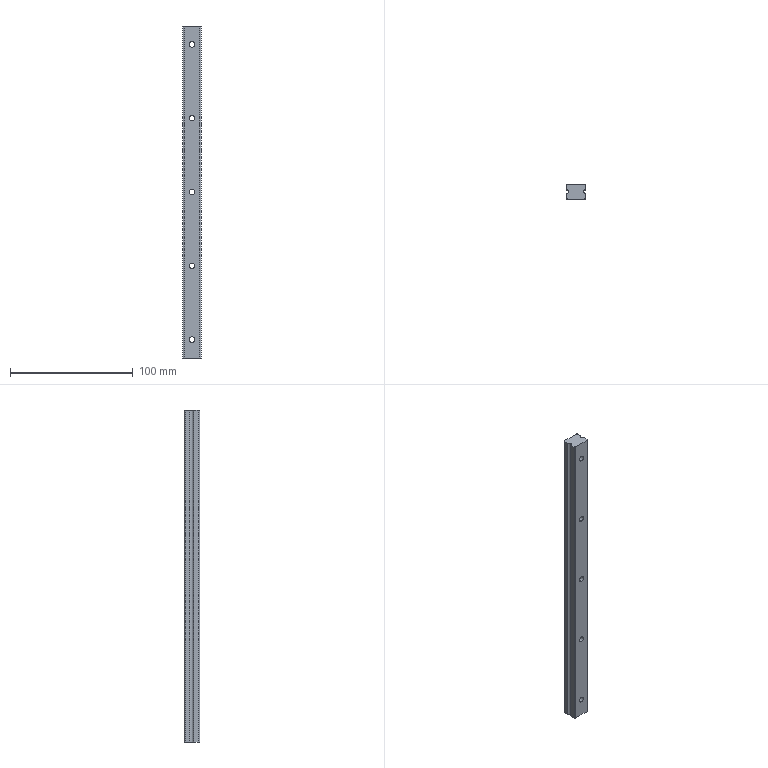Part | STEP file | Guide rail SSR15XW1SSC1+270LY | 1 solid | 40 faces | box 15 x 12.5 x 270 mm | volume 46741 mm3 | cylinder 27 | plane 13 | commonest cylinder face diameters 4.5 x10 7.5 x10 2 x4 3 x3